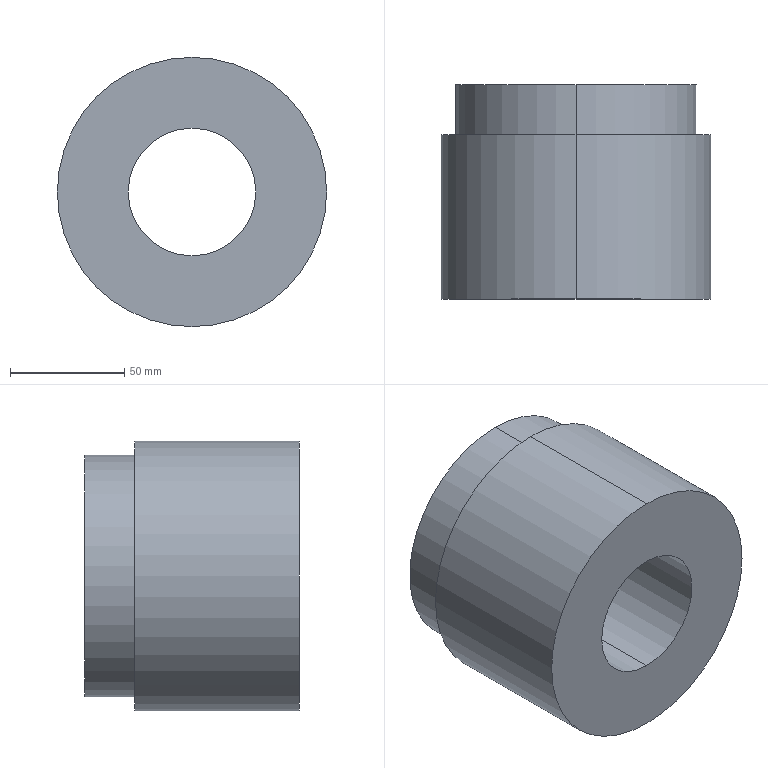Part | SolidWorks | features Extrusion 1, ICE 1 | 1 solid | 9 faces | box 118 x 94 x 118 mm | volume 750005 mm3 | cylinder 6 | plane 3 | commonest cylinder face diameters 56 x2 106 x2 118 x2
STEP:
#1=CARTESIAN_POINT('',(0.,72.,53.));
#2=VERTEX_POINT('',#1);
#3=CARTESIAN_POINT('',(0.,72.,-53.));
#4=VERTEX_POINT('',#3);
#5=CARTESIAN_POINT('',(0.,72.,0.));
#6=DIRECTION('',(0.,1.,0.));
#7=DIRECTION('',(0.,0.,1.));
#8=AXIS2_PLACEMENT_3D('',#5,#6,#7);
#9=CIRCLE('',#8,53.);
#10=EDGE_CURVE('',#2,#4,#9,.T.);
#11=ORIENTED_EDGE('',*,*,#10,.T.);
#12=CARTESIAN_POINT('',(0.,94.,-53.));
#13=VERTEX_POINT('',#12);
#14=CARTESIAN_POINT('',(0.,72.,-53.));
#15=DIRECTION('',(0.,1.,0.));
#16=VECTOR('',#15,1000.);
#17=LINE('',#14,#16);
#18=EDGE_CURVE('',#4,#13,#17,.T.);
#19=ORIENTED_EDGE('',*,*,#18,.T.);
#20=CARTESIAN_POINT('',(0.,94.,53.));
#21=VERTEX_POINT('',#20);
#22=CARTESIAN_POINT('',(0.,94.,0.));
#23=DIRECTION('',(0.,1.,0.));
#24=DIRECTION('',(0.,0.,1.));
#25=AXIS2_PLACEMENT_3D('',#22,#23,#24);
#26=CIRCLE('',#25,53.);
#27=EDGE_CURVE('',#21,#13,#26,.T.);
#28=ORIENTED_EDGE('',*,*,#27,.F.);
#29=CARTESIAN_POINT('',(0.,72.,53.));
#30=DIRECTION('',(0.,1.,0.));
#31=VECTOR('',#30,1000.);
#32=LINE('',#29,#31);
#33=EDGE_CURVE('',#2,#21,#32,.T.);
#34=ORIENTED_EDGE('',*,*,#33,.F.);
#35=EDGE_LOOP('',(#11,#19,#28,#34));
#36=FACE_OUTER_BOUND('',#35,.T.);
#37=CARTESIAN_POINT('',(0.,72.,0.));
#38=DIRECTION('',(0.,1.,0.));
#39=DIRECTION('',(0.,0.,1.));
#40=AXIS2_PLACEMENT_3D('',#37,#38,#39);
#41=CYLINDRICAL_SURFACE('',#40,53.);
#42=ADVANCED_FACE('',(#36),#41,.T.);
#43=CARTESIAN_POINT('',(0.,94.,-28.));
#44=VERTEX_POINT('',#43);
#45=CARTESIAN_POINT('',(0.,94.,28.));
#46=VERTEX_POINT('',#45);
#47=CARTESIAN_POINT('',(0.,94.,0.));
#48=DIRECTION('',(0.,1.,0.));
#49=DIRECTION('',(0.,0.,1.));
#50=AXIS2_PLACEMENT_3D('',#47,#48,#49);
#51=CIRCLE('',#50,28.);
#52=EDGE_CURVE('',#44,#46,#51,.T.);
#53=ORIENTED_EDGE('',*,*,#52,.T.);
#54=CARTESIAN_POINT('',(0.,0.,28.));
#55=VERTEX_POINT('',#54);
#56=CARTESIAN_POINT('',(0.,94.,28.));
#57=DIRECTION('',(0.,-1.,0.));
#58=VECTOR('',#57,1000.);
#59=LINE('',#56,#58);
#60=EDGE_CURVE('',#46,#55,#59,.T.);
#61=ORIENTED_EDGE('',*,*,#60,.T.);
#62=CARTESIAN_POINT('',(0.,0.,-28.));
#63=VERTEX_POINT('',#62);
#64=CARTESIAN_POINT('',(0.,0.,0.));
#65=DIRECTION('',(0.,1.,0.));
#66=DIRECTION('',(0.,0.,1.));
#67=AXIS2_PLACEMENT_3D('',#64,#65,#66);
#68=CIRCLE('',#67,28.);
#69=EDGE_CURVE('',#63,#55,#68,.T.);
#70=ORIENTED_EDGE('',*,*,#69,.F.);
#71=CARTESIAN_POINT('',(0.,94.,-28.));
#72=DIRECTION('',(0.,-1.,0.));
#73=VECTOR('',#72,1000.);
#74=LINE('',#71,#73);
#75=EDGE_CURVE('',#44,#63,#74,.T.);
#76=ORIENTED_EDGE('',*,*,#75,.F.);
#77=EDGE_LOOP('',(#53,#61,#70,#76));
#78=FACE_OUTER_BOUND('',#77,.T.);
#79=CARTESIAN_POINT('',(0.,94.,0.));
#80=DIRECTION('',(0.,-1.,0.));
#81=DIRECTION('',(0.,0.,-1.));
#82=AXIS2_PLACEMENT_3D('',#79,#80,#81);
#83=CYLINDRICAL_SURFACE('',#82,28.);
#84=ADVANCED_FACE('',(#78),#83,.F.);
#85=CARTESIAN_POINT('',(0.,72.,59.));
#86=VERTEX_POINT('',#85);
#87=CARTESIAN_POINT('',(0.,72.,-59.));
#88=VERTEX_POINT('',#87);
#89=CARTESIAN_POINT('',(0.,72.,0.));
#90=DIRECTION('',(0.,1.,0.));
#91=DIRECTION('',(0.,0.,1.));
#92=AXIS2_PLACEMENT_3D('',#89,#90,#91);
#93=CIRCLE('',#92,59.);
#94=EDGE_CURVE('',#86,#88,#93,.T.);
#95=ORIENTED_EDGE('',*,*,#94,.F.);
#96=CARTESIAN_POINT('',(0.,0.,59.));
#97=VERTEX_POINT('',#96);
#98=CARTESIAN_POINT('',(0.,94.,59.));
#99=DIRECTION('',(0.,-1.,0.));
#100=VECTOR('',#99,1000.);
#101=LINE('',#98,#100);
#102=EDGE_CURVE('',#86,#97,#101,.T.);
#103=ORIENTED_EDGE('',*,*,#102,.T.);
#104=CARTESIAN_POINT('',(0.,0.,-59.));
#105=VERTEX_POINT('',#104);
#106=CARTESIAN_POINT('',(0.,0.,0.));
#107=DIRECTION('',(0.,1.,0.));
#108=DIRECTION('',(0.,0.,1.));
#109=AXIS2_PLACEMENT_3D('',#106,#107,#108);
#110=CIRCLE('',#109,59.);
#111=EDGE_CURVE('',#97,#105,#110,.T.);
#112=ORIENTED_EDGE('',*,*,#111,.T.);
#113=CARTESIAN_POINT('',(0.,94.,-59.));
#114=DIRECTION('',(0.,-1.,0.));
#115=VECTOR('',#114,1000.);
#116=LINE('',#113,#115);
#117=EDGE_CURVE('',#88,#105,#116,.T.);
#118=ORIENTED_EDGE('',*,*,#117,.F.);
#119=EDGE_LOOP('',(#95,#103,#112,#118));
#120=FACE_OUTER_BOUND('',#119,.T.);
#121=CARTESIAN_POINT('',(0.,94.,0.));
#122=DIRECTION('',(0.,-1.,0.));
#123=DIRECTION('',(0.,0.,-1.));
#124=AXIS2_PLACEMENT_3D('',#121,#122,#123);
#125=CYLINDRICAL_SURFACE('',#124,59.);
#126=ADVANCED_FACE('',(#120),#125,.T.);
#127=ORIENTED_EDGE('',*,*,#52,.F.);
#128=CARTESIAN_POINT('',(0.,94.,0.));
#129=DIRECTION('',(0.,1.,0.));
#130=DIRECTION('',(0.,0.,1.));
#131=AXIS2_PLACEMENT_3D('',#128,#129,#130);
#132=CIRCLE('',#131,28.);
#133=EDGE_CURVE('',#46,#44,#132,.T.);
#134=ORIENTED_EDGE('',*,*,#133,.F.);
#135=EDGE_LOOP('',(#127,#134));
#136=FACE_BOUND('',#135,.T.);
#137=ORIENTED_EDGE('',*,*,#27,.T.);
#138=CARTESIAN_POINT('',(0.,94.,0.));
#139=DIRECTION('',(0.,1.,0.));
#140=DIRECTION('',(0.,0.,1.));
#141=AXIS2_PLACEMENT_3D('',#138,#139,#140);
#142=CIRCLE('',#141,53.);
#143=EDGE_CURVE('',#13,#21,#142,.T.);
#144=ORIENTED_EDGE('',*,*,#143,.T.);
#145=EDGE_LOOP('',(#137,#144));
#146=FACE_OUTER_BOUND('',#145,.T.);
#147=CARTESIAN_POINT('',(0.,94.,0.));
#148=DIRECTION('',(0.,1.,0.));
#149=DIRECTION('',(0.,0.,1.));
#150=AXIS2_PLACEMENT_3D('',#147,#148,#149);
#151=PLANE('',#150);
#152=ADVANCED_FACE('',(#136,#146),#151,.T.);
#153=ORIENTED_EDGE('',*,*,#102,.F.);
#154=CARTESIAN_POINT('',(0.,72.,0.));
#155=DIRECTION('',(0.,1.,0.));
#156=DIRECTION('',(0.,0.,1.));
#157=AXIS2_PLACEMENT_3D('',#154,#155,#156);
#158=CIRCLE('',#157,59.);
#159=EDGE_CURVE('',#88,#86,#158,.T.);
#160=ORIENTED_EDGE('',*,*,#159,.F.);
#161=ORIENTED_EDGE('',*,*,#117,.T.);
#162=CARTESIAN_POINT('',(0.,0.,0.));
#163=DIRECTION('',(0.,1.,0.));
#164=DIRECTION('',(0.,0.,1.));
#165=AXIS2_PLACEMENT_3D('',#162,#163,#164);
#166=CIRCLE('',#165,59.);
#167=EDGE_CURVE('',#105,#97,#166,.T.);
#168=ORIENTED_EDGE('',*,*,#167,.T.);
#169=EDGE_LOOP('',(#153,#160,#161,#168));
#170=FACE_OUTER_BOUND('',#169,.T.);
#171=CARTESIAN_POINT('',(0.,94.,0.));
#172=DIRECTION('',(0.,-1.,0.));
#173=DIRECTION('',(0.,0.,-1.));
#174=AXIS2_PLACEMENT_3D('',#171,#172,#173);
#175=CYLINDRICAL_SURFACE('',#174,59.);
#176=ADVANCED_FACE('',(#170),#175,.T.);
#177=ORIENTED_EDGE('',*,*,#167,.F.);
#178=ORIENTED_EDGE('',*,*,#111,.F.);
#179=EDGE_LOOP('',(#177,#178));
#180=FACE_OUTER_BOUND('',#179,.T.);
#181=ORIENTED_EDGE('',*,*,#69,.T.);
#182=CARTESIAN_POINT('',(0.,0.,0.));
#183=DIRECTION('',(0.,1.,0.));
#184=DIRECTION('',(0.,0.,1.));
#185=AXIS2_PLACEMENT_3D('',#182,#183,#184);
#186=CIRCLE('',#185,28.);
#187=EDGE_CURVE('',#55,#63,#186,.T.);
#188=ORIENTED_EDGE('',*,*,#187,.T.);
#189=EDGE_LOOP('',(#181,#188));
#190=FACE_BOUND('',#189,.T.);
#191=CARTESIAN_POINT('',(0.,0.,0.));
#192=DIRECTION('',(0.,1.,0.));
#193=DIRECTION('',(0.,0.,1.));
#194=AXIS2_PLACEMENT_3D('',#191,#192,#193);
#195=PLANE('',#194);
#196=ADVANCED_FACE('',(#180,#190),#195,.F.);
#197=ORIENTED_EDGE('',*,*,#60,.F.);
#198=ORIENTED_EDGE('',*,*,#133,.T.);
#199=ORIENTED_EDGE('',*,*,#75,.T.);
#200=ORIENTED_EDGE('',*,*,#187,.F.);
#201=EDGE_LOOP('',(#197,#198,#199,#200));
#202=FACE_OUTER_BOUND('',#201,.T.);
#203=CARTESIAN_POINT('',(0.,94.,0.));
#204=DIRECTION('',(0.,-1.,0.));
#205=DIRECTION('',(0.,0.,-1.));
#206=AXIS2_PLACEMENT_3D('',#203,#204,#205);
#207=CYLINDRICAL_SURFACE('',#206,28.);
#208=ADVANCED_FACE('',(#202),#207,.F.);
#209=ORIENTED_EDGE('',*,*,#10,.F.);
#210=CARTESIAN_POINT('',(0.,72.,0.));
#211=DIRECTION('',(0.,1.,0.));
#212=DIRECTION('',(0.,0.,1.));
#213=AXIS2_PLACEMENT_3D('',#210,#211,#212);
#214=CIRCLE('',#213,53.);
#215=EDGE_CURVE('',#4,#2,#214,.T.);
#216=ORIENTED_EDGE('',*,*,#215,.F.);
#217=EDGE_LOOP('',(#209,#216));
#218=FACE_BOUND('',#217,.T.);
#219=ORIENTED_EDGE('',*,*,#159,.T.);
#220=ORIENTED_EDGE('',*,*,#94,.T.);
#221=EDGE_LOOP('',(#219,#220));
#222=FACE_OUTER_BOUND('',#221,.T.);
#223=CARTESIAN_POINT('',(0.,72.,0.));
#224=DIRECTION('',(0.,1.,0.));
#225=DIRECTION('',(0.,0.,1.));
#226=AXIS2_PLACEMENT_3D('',#223,#224,#225);
#227=PLANE('',#226);
#228=ADVANCED_FACE('',(#218,#222),#227,.T.);
#229=ORIENTED_EDGE('',*,*,#18,.F.);
#230=ORIENTED_EDGE('',*,*,#215,.T.);
#231=ORIENTED_EDGE('',*,*,#33,.T.);
#232=ORIENTED_EDGE('',*,*,#143,.F.);
#233=EDGE_LOOP('',(#229,#230,#231,#232));
#234=FACE_OUTER_BOUND('',#233,.T.);
#235=CARTESIAN_POINT('',(0.,72.,0.));
#236=DIRECTION('',(0.,1.,0.));
#237=DIRECTION('',(0.,0.,1.));
#238=AXIS2_PLACEMENT_3D('',#235,#236,#237);
#239=CYLINDRICAL_SURFACE('',#238,53.);
#240=ADVANCED_FACE('',(#234),#239,.T.);
#241=CLOSED_SHELL('',(#42,#84,#126,#152,#176,#196,#208,#228,#240));
#242=MANIFOLD_SOLID_BREP('',#241);
#243=CARTESIAN_POINT('',(0.,0.,0.));
#244=DIRECTION('',(0.,0.,1.));
#245=DIRECTION('',(1.,0.,0.));
#246=AXIS2_PLACEMENT_3D('',#243,#244,#245);
#247=(LENGTH_UNIT()NAMED_UNIT(*)SI_UNIT(.MILLI.,.METRE.));
#248=UNCERTAINTY_MEASURE_WITH_UNIT(LENGTH_MEASURE(0.00001),#247,'','');
#249=(NAMED_UNIT(*)PLANE_ANGLE_UNIT()SI_UNIT($,.RADIAN.));
#250=(NAMED_UNIT(*)SI_UNIT($,.STERADIAN.)SOLID_ANGLE_UNIT());
#251=(GEOMETRIC_REPRESENTATION_CONTEXT(3)GLOBAL_UNCERTAINTY_ASSIGNED_CONTEXT((#248))GLOBAL_UNIT_ASSIGNED_CONTEXT((#247,#249,#250))REPRESENTATION_CONTEXT('',''));
#252=ADVANCED_BREP_SHAPE_REPRESENTATION('',(#242,#246),#251);